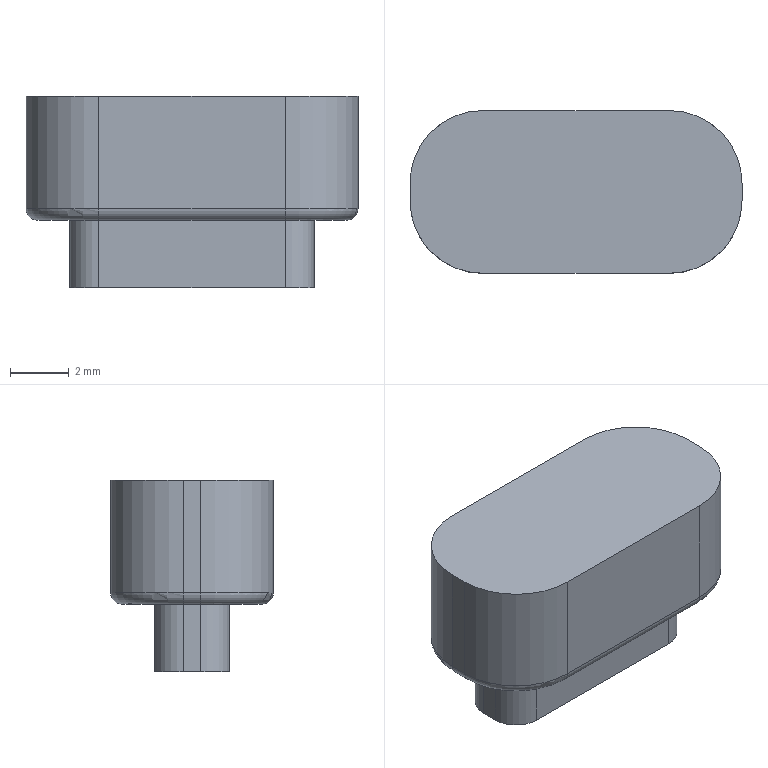Part | Creo | 1 solid | 27 faces | box 11.34 x 5.56 x 6.53 mm | volume 290.585 mm3 | cylinder 12 | plane 11 | torus 4 | commonest cylinder face diameters 0.8 x4 1.96 x4 4.96 x4
STEP:
#1=CARTESIAN_POINT('',(0.,0.,0.));
#2=DIRECTION('',(0.,0.,1.));
#3=DIRECTION('',(1.,0.,0.));
#4=AXIS2_PLACEMENT_3D('',#1,#2,#3);
#5=CARTESIAN_POINT('',(14.105,3.73,-58.15));
#6=VERTEX_POINT('',#5);
#7=CARTESIAN_POINT('',(7.725,3.73,-58.15));
#8=VERTEX_POINT('',#7);
#9=CARTESIAN_POINT('',(14.105,3.73,-58.15));
#10=DIRECTION('',(-1.,0.,0.));
#11=VECTOR('',#10,6.38);
#12=LINE('',#9,#11);
#13=EDGE_CURVE('',#6,#8,#12,.T.);
#14=ORIENTED_EDGE('',*,*,#13,.F.);
#15=CARTESIAN_POINT('',(14.105,3.73,-54.32));
#16=VERTEX_POINT('',#15);
#17=CARTESIAN_POINT('',(14.105,3.73,-54.32));
#18=DIRECTION('',(0.,0.,-1.));
#19=VECTOR('',#18,3.83);
#20=LINE('',#17,#19);
#21=EDGE_CURVE('',#16,#6,#20,.T.);
#22=ORIENTED_EDGE('',*,*,#21,.F.);
#23=CARTESIAN_POINT('',(7.725,3.73,-54.32));
#24=VERTEX_POINT('',#23);
#25=CARTESIAN_POINT('',(14.105,3.73,-54.32));
#26=DIRECTION('',(-1.,0.,0.));
#27=VECTOR('',#26,6.38);
#28=LINE('',#25,#27);
#29=EDGE_CURVE('',#16,#24,#28,.T.);
#30=ORIENTED_EDGE('',*,*,#29,.T.);
#31=CARTESIAN_POINT('',(7.725,3.73,-58.15));
#32=DIRECTION('',(0.,0.,1.));
#33=VECTOR('',#32,3.83);
#34=LINE('',#31,#33);
#35=EDGE_CURVE('',#8,#24,#34,.T.);
#36=ORIENTED_EDGE('',*,*,#35,.F.);
#37=EDGE_LOOP('',(#14,#22,#30,#36));
#38=FACE_OUTER_BOUND('',#37,.F.);
#39=CARTESIAN_POINT('',(14.105,3.73,-58.55));
#40=DIRECTION('',(0.,1.,0.));
#41=DIRECTION('',(-1.,0.,0.));
#42=AXIS2_PLACEMENT_3D('',#39,#40,#41);
#43=PLANE('',#42);
#44=ADVANCED_FACE('',(#38),#43,.T.);
#45=CARTESIAN_POINT('',(7.725,3.33,-58.55));
#46=VERTEX_POINT('',#45);
#47=CARTESIAN_POINT('',(14.105,3.33,-58.55));
#48=VERTEX_POINT('',#47);
#49=CARTESIAN_POINT('',(7.725,3.33,-58.55));
#50=DIRECTION('',(1.,0.,0.));
#51=VECTOR('',#50,6.38);
#52=LINE('',#49,#51);
#53=EDGE_CURVE('',#46,#48,#52,.T.);
#54=ORIENTED_EDGE('',*,*,#53,.T.);
#55=CARTESIAN_POINT('',(14.105,3.33,-58.15));
#56=DIRECTION('',(-1.,0.,0.));
#57=DIRECTION('',(0.,1.,0.));
#58=AXIS2_PLACEMENT_3D('',#55,#56,#57);
#59=CIRCLE('',#58,0.4);
#60=EDGE_CURVE('',#6,#48,#59,.T.);
#61=ORIENTED_EDGE('',*,*,#60,.F.);
#62=ORIENTED_EDGE('',*,*,#13,.T.);
#63=CARTESIAN_POINT('',(7.725,3.33,-58.15));
#64=DIRECTION('',(1.,0.,0.));
#65=DIRECTION('',(0.,0.,-1.));
#66=AXIS2_PLACEMENT_3D('',#63,#64,#65);
#67=CIRCLE('',#66,0.4);
#68=EDGE_CURVE('',#46,#8,#67,.T.);
#69=ORIENTED_EDGE('',*,*,#68,.F.);
#70=EDGE_LOOP('',(#54,#61,#62,#69));
#71=FACE_OUTER_BOUND('',#70,.F.);
#72=CARTESIAN_POINT('',(7.681,3.33,-58.15));
#73=DIRECTION('',(1.,0.,0.));
#74=DIRECTION('',(0.,0.,-1.));
#75=AXIS2_PLACEMENT_3D('',#72,#73,#74);
#76=CYLINDRICAL_SURFACE('',#75,0.4);
#77=ADVANCED_FACE('',(#71),#76,.T.);
#78=CARTESIAN_POINT('',(16.185,1.25,-58.55));
#79=VERTEX_POINT('',#78);
#80=CARTESIAN_POINT('',(14.105,1.25,-58.55));
#81=DIRECTION('',(0.,0.,1.));
#82=DIRECTION('',(1.,0.,0.));
#83=AXIS2_PLACEMENT_3D('',#80,#81,#82);
#84=CIRCLE('',#83,2.08);
#85=EDGE_CURVE('',#79,#48,#84,.T.);
#86=ORIENTED_EDGE('',*,*,#85,.T.);
#87=ORIENTED_EDGE('',*,*,#53,.F.);
#88=CARTESIAN_POINT('',(5.645,1.25,-58.55));
#89=VERTEX_POINT('',#88);
#90=CARTESIAN_POINT('',(7.725,1.25,-58.55));
#91=DIRECTION('',(0.,0.,1.));
#92=DIRECTION('',(0.,1.,0.));
#93=AXIS2_PLACEMENT_3D('',#90,#91,#92);
#94=CIRCLE('',#93,2.08);
#95=EDGE_CURVE('',#46,#89,#94,.T.);
#96=ORIENTED_EDGE('',*,*,#95,.T.);
#97=CARTESIAN_POINT('',(5.645,0.65,-58.55));
#98=VERTEX_POINT('',#97);
#99=CARTESIAN_POINT('',(5.645,0.65,-58.55));
#100=DIRECTION('',(0.,1.,0.));
#101=VECTOR('',#100,0.6);
#102=LINE('',#99,#101);
#103=EDGE_CURVE('',#98,#89,#102,.T.);
#104=ORIENTED_EDGE('',*,*,#103,.F.);
#105=CARTESIAN_POINT('',(7.725,-1.43,-58.55));
#106=VERTEX_POINT('',#105);
#107=CARTESIAN_POINT('',(7.725,0.65,-58.55));
#108=DIRECTION('',(0.,0.,1.));
#109=DIRECTION('',(-1.,0.,0.));
#110=AXIS2_PLACEMENT_3D('',#107,#108,#109);
#111=CIRCLE('',#110,2.08);
#112=EDGE_CURVE('',#98,#106,#111,.T.);
#113=ORIENTED_EDGE('',*,*,#112,.T.);
#114=CARTESIAN_POINT('',(14.105,-1.43,-58.55));
#115=VERTEX_POINT('',#114);
#116=CARTESIAN_POINT('',(14.105,-1.43,-58.55));
#117=DIRECTION('',(-1.,0.,0.));
#118=VECTOR('',#117,6.38);
#119=LINE('',#116,#118);
#120=EDGE_CURVE('',#115,#106,#119,.T.);
#121=ORIENTED_EDGE('',*,*,#120,.F.);
#122=CARTESIAN_POINT('',(16.185,0.65,-58.55));
#123=VERTEX_POINT('',#122);
#124=CARTESIAN_POINT('',(14.105,0.65,-58.55));
#125=DIRECTION('',(0.,0.,1.));
#126=DIRECTION('',(0.,-1.,0.));
#127=AXIS2_PLACEMENT_3D('',#124,#125,#126);
#128=CIRCLE('',#127,2.08);
#129=EDGE_CURVE('',#115,#123,#128,.T.);
#130=ORIENTED_EDGE('',*,*,#129,.T.);
#131=CARTESIAN_POINT('',(16.185,1.25,-58.55));
#132=DIRECTION('',(0.,-1.,0.));
#133=VECTOR('',#132,0.6);
#134=LINE('',#131,#133);
#135=EDGE_CURVE('',#79,#123,#134,.T.);
#136=ORIENTED_EDGE('',*,*,#135,.F.);
#137=EDGE_LOOP('',(#86,#87,#96,#104,#113,#121,#130,#136));
#138=FACE_OUTER_BOUND('',#137,.F.);
#139=CARTESIAN_POINT('',(15.085,0.65,-58.55));
#140=VERTEX_POINT('',#139);
#141=CARTESIAN_POINT('',(14.105,-0.33,-58.55));
#142=VERTEX_POINT('',#141);
#143=CARTESIAN_POINT('',(14.105,0.65,-58.55));
#144=DIRECTION('',(0.,0.,-1.));
#145=DIRECTION('',(1.,0.,0.));
#146=AXIS2_PLACEMENT_3D('',#143,#144,#145);
#147=CIRCLE('',#146,0.98);
#148=EDGE_CURVE('',#140,#142,#147,.T.);
#149=ORIENTED_EDGE('',*,*,#148,.T.);
#150=CARTESIAN_POINT('',(7.725,-0.33,-58.55));
#151=VERTEX_POINT('',#150);
#152=CARTESIAN_POINT('',(7.725,-0.33,-58.55));
#153=DIRECTION('',(1.,0.,0.));
#154=VECTOR('',#153,6.38);
#155=LINE('',#152,#154);
#156=EDGE_CURVE('',#151,#142,#155,.T.);
#157=ORIENTED_EDGE('',*,*,#156,.F.);
#158=CARTESIAN_POINT('',(6.745,0.65,-58.55));
#159=VERTEX_POINT('',#158);
#160=CARTESIAN_POINT('',(7.725,0.65,-58.55));
#161=DIRECTION('',(0.,0.,-1.));
#162=DIRECTION('',(0.,-1.,0.));
#163=AXIS2_PLACEMENT_3D('',#160,#161,#162);
#164=CIRCLE('',#163,0.98);
#165=EDGE_CURVE('',#151,#159,#164,.T.);
#166=ORIENTED_EDGE('',*,*,#165,.T.);
#167=CARTESIAN_POINT('',(6.745,1.25,-58.55));
#168=VERTEX_POINT('',#167);
#169=CARTESIAN_POINT('',(6.745,1.25,-58.55));
#170=DIRECTION('',(0.,-1.,0.));
#171=VECTOR('',#170,0.6);
#172=LINE('',#169,#171);
#173=EDGE_CURVE('',#168,#159,#172,.T.);
#174=ORIENTED_EDGE('',*,*,#173,.F.);
#175=CARTESIAN_POINT('',(7.725,2.23,-58.55));
#176=VERTEX_POINT('',#175);
#177=CARTESIAN_POINT('',(7.725,1.25,-58.55));
#178=DIRECTION('',(0.,0.,-1.));
#179=DIRECTION('',(-1.,0.,0.));
#180=AXIS2_PLACEMENT_3D('',#177,#178,#179);
#181=CIRCLE('',#180,0.98);
#182=EDGE_CURVE('',#168,#176,#181,.T.);
#183=ORIENTED_EDGE('',*,*,#182,.T.);
#184=CARTESIAN_POINT('',(14.105,2.23,-58.55));
#185=VERTEX_POINT('',#184);
#186=CARTESIAN_POINT('',(14.105,2.23,-58.55));
#187=DIRECTION('',(-1.,0.,0.));
#188=VECTOR('',#187,6.38);
#189=LINE('',#186,#188);
#190=EDGE_CURVE('',#185,#176,#189,.T.);
#191=ORIENTED_EDGE('',*,*,#190,.F.);
#192=CARTESIAN_POINT('',(15.085,1.25,-58.55));
#193=VERTEX_POINT('',#192);
#194=CARTESIAN_POINT('',(14.105,1.25,-58.55));
#195=DIRECTION('',(0.,0.,-1.));
#196=DIRECTION('',(0.,1.,0.));
#197=AXIS2_PLACEMENT_3D('',#194,#195,#196);
#198=CIRCLE('',#197,0.98);
#199=EDGE_CURVE('',#185,#193,#198,.T.);
#200=ORIENTED_EDGE('',*,*,#199,.T.);
#201=CARTESIAN_POINT('',(15.085,0.65,-58.55));
#202=DIRECTION('',(0.,1.,0.));
#203=VECTOR('',#202,0.6);
#204=LINE('',#201,#203);
#205=EDGE_CURVE('',#140,#193,#204,.T.);
#206=ORIENTED_EDGE('',*,*,#205,.F.);
#207=EDGE_LOOP('',(#149,#157,#166,#174,#183,#191,#200,#206));
#208=FACE_BOUND('',#207,.F.);
#209=CARTESIAN_POINT('',(0.,0.,-58.55));
#210=DIRECTION('',(0.,0.,1.));
#211=DIRECTION('',(1.,0.,0.));
#212=AXIS2_PLACEMENT_3D('',#209,#210,#211);
#213=PLANE('',#212);
#214=ADVANCED_FACE('',(#138,#208),#213,.F.);
#215=ORIENTED_EDGE('',*,*,#85,.F.);
#216=CARTESIAN_POINT('',(16.585,1.25,-58.15));
#217=VERTEX_POINT('',#216);
#218=CARTESIAN_POINT('',(16.185,1.25,-58.15));
#219=DIRECTION('',(0.,-1.,0.));
#220=DIRECTION('',(0.,0.,-1.));
#221=AXIS2_PLACEMENT_3D('',#218,#219,#220);
#222=CIRCLE('',#221,0.4);
#223=EDGE_CURVE('',#79,#217,#222,.T.);
#224=ORIENTED_EDGE('',*,*,#223,.T.);
#225=CARTESIAN_POINT('',(14.105,1.25,-58.15));
#226=DIRECTION('',(0.,0.,1.));
#227=DIRECTION('',(1.,0.,0.));
#228=AXIS2_PLACEMENT_3D('',#225,#226,#227);
#229=CIRCLE('',#228,2.48);
#230=EDGE_CURVE('',#217,#6,#229,.T.);
#231=ORIENTED_EDGE('',*,*,#230,.T.);
#232=ORIENTED_EDGE('',*,*,#60,.T.);
#233=EDGE_LOOP('',(#215,#224,#231,#232));
#234=FACE_OUTER_BOUND('',#233,.F.);
#235=CARTESIAN_POINT('',(14.105,1.25,-58.15));
#236=DIRECTION('',(0.,0.,1.));
#237=DIRECTION('',(-0.01768,0.9998,0.));
#238=AXIS2_PLACEMENT_3D('',#235,#236,#237);
#239=TOROIDAL_SURFACE('',#238,2.08,0.4);
#240=ADVANCED_FACE('',(#234),#239,.T.);
#241=ORIENTED_EDGE('',*,*,#135,.T.);
#242=CARTESIAN_POINT('',(16.585,0.65,-58.15));
#243=VERTEX_POINT('',#242);
#244=CARTESIAN_POINT('',(16.185,0.65,-58.15));
#245=DIRECTION('',(0.,1.,0.));
#246=DIRECTION('',(1.,0.,0.));
#247=AXIS2_PLACEMENT_3D('',#244,#245,#246);
#248=CIRCLE('',#247,0.4);
#249=EDGE_CURVE('',#243,#123,#248,.T.);
#250=ORIENTED_EDGE('',*,*,#249,.F.);
#251=CARTESIAN_POINT('',(16.585,0.65,-58.15));
#252=DIRECTION('',(0.,1.,0.));
#253=VECTOR('',#252,0.6);
#254=LINE('',#251,#253);
#255=EDGE_CURVE('',#243,#217,#254,.T.);
#256=ORIENTED_EDGE('',*,*,#255,.T.);
#257=ORIENTED_EDGE('',*,*,#223,.F.);
#258=EDGE_LOOP('',(#241,#250,#256,#257));
#259=FACE_OUTER_BOUND('',#258,.F.);
#260=CARTESIAN_POINT('',(16.185,1.294,-58.15));
#261=DIRECTION('',(0.,-1.,0.));
#262=DIRECTION('',(0.,0.,-1.));
#263=AXIS2_PLACEMENT_3D('',#260,#261,#262);
#264=CYLINDRICAL_SURFACE('',#263,0.4);
#265=ADVANCED_FACE('',(#259),#264,.T.);
#266=ORIENTED_EDGE('',*,*,#129,.F.);
#267=CARTESIAN_POINT('',(14.105,-1.83,-58.15));
#268=VERTEX_POINT('',#267);
#269=CARTESIAN_POINT('',(14.105,-1.43,-58.15));
#270=DIRECTION('',(-1.,0.,0.));
#271=DIRECTION('',(0.,0.,-1.));
#272=AXIS2_PLACEMENT_3D('',#269,#270,#271);
#273=CIRCLE('',#272,0.4);
#274=EDGE_CURVE('',#115,#268,#273,.T.);
#275=ORIENTED_EDGE('',*,*,#274,.T.);
#276=CARTESIAN_POINT('',(14.105,0.65,-58.15));
#277=DIRECTION('',(0.,0.,1.));
#278=DIRECTION('',(0.,-1.,0.));
#279=AXIS2_PLACEMENT_3D('',#276,#277,#278);
#280=CIRCLE('',#279,2.48);
#281=EDGE_CURVE('',#268,#243,#280,.T.);
#282=ORIENTED_EDGE('',*,*,#281,.T.);
#283=ORIENTED_EDGE('',*,*,#249,.T.);
#284=EDGE_LOOP('',(#266,#275,#282,#283));
#285=FACE_OUTER_BOUND('',#284,.F.);
#286=CARTESIAN_POINT('',(14.105,0.65,-58.15));
#287=DIRECTION('',(0.,0.,1.));
#288=DIRECTION('',(0.9998,0.01768,0.));
#289=AXIS2_PLACEMENT_3D('',#286,#287,#288);
#290=TOROIDAL_SURFACE('',#289,2.08,0.4);
#291=ADVANCED_FACE('',(#285),#290,.T.);
#292=ORIENTED_EDGE('',*,*,#120,.T.);
#293=CARTESIAN_POINT('',(7.725,-1.83,-58.15));
#294=VERTEX_POINT('',#293);
#295=CARTESIAN_POINT('',(7.725,-1.43,-58.15));
#296=DIRECTION('',(1.,0.,0.));
#297=DIRECTION('',(0.,-1.,0.));
#298=AXIS2_PLACEMENT_3D('',#295,#296,#297);
#299=CIRCLE('',#298,0.4);
#300=EDGE_CURVE('',#294,#106,#299,.T.);
#301=ORIENTED_EDGE('',*,*,#300,.F.);
#302=CARTESIAN_POINT('',(7.725,-1.83,-58.15));
#303=DIRECTION('',(1.,0.,0.));
#304=VECTOR('',#303,6.38);
#305=LINE('',#302,#304);
#306=EDGE_CURVE('',#294,#268,#305,.T.);
#307=ORIENTED_EDGE('',*,*,#306,.T.);
#308=ORIENTED_EDGE('',*,*,#274,.F.);
#309=EDGE_LOOP('',(#292,#301,#307,#308));
#310=FACE_OUTER_BOUND('',#309,.F.);
#311=CARTESIAN_POINT('',(14.149,-1.43,-58.15));
#312=DIRECTION('',(-1.,0.,0.));
#313=DIRECTION('',(0.,0.,-1.));
#314=AXIS2_PLACEMENT_3D('',#311,#312,#313);
#315=CYLINDRICAL_SURFACE('',#314,0.4);
#316=ADVANCED_FACE('',(#310),#315,.T.);
#317=ORIENTED_EDGE('',*,*,#112,.F.);
#318=CARTESIAN_POINT('',(5.245,0.65,-58.15));
#319=VERTEX_POINT('',#318);
#320=CARTESIAN_POINT('',(5.645,0.65,-58.15));
#321=DIRECTION('',(0.,1.,0.));
#322=DIRECTION('',(0.,0.,-1.));
#323=AXIS2_PLACEMENT_3D('',#320,#321,#322);
#324=CIRCLE('',#323,0.4);
#325=EDGE_CURVE('',#98,#319,#324,.T.);
#326=ORIENTED_EDGE('',*,*,#325,.T.);
#327=CARTESIAN_POINT('',(7.725,0.65,-58.15));
#328=DIRECTION('',(0.,0.,1.));
#329=DIRECTION('',(-1.,0.,0.));
#330=AXIS2_PLACEMENT_3D('',#327,#328,#329);
#331=CIRCLE('',#330,2.48);
#332=EDGE_CURVE('',#319,#294,#331,.T.);
#333=ORIENTED_EDGE('',*,*,#332,.T.);
#334=ORIENTED_EDGE('',*,*,#300,.T.);
#335=EDGE_LOOP('',(#317,#326,#333,#334));
#336=FACE_OUTER_BOUND('',#335,.F.);
#337=CARTESIAN_POINT('',(7.725,0.65,-58.15));
#338=DIRECTION('',(0.,0.,1.));
#339=DIRECTION('',(0.01768,-0.9998,0.));
#340=AXIS2_PLACEMENT_3D('',#337,#338,#339);
#341=TOROIDAL_SURFACE('',#340,2.08,0.4);
#342=ADVANCED_FACE('',(#336),#341,.T.);
#343=ORIENTED_EDGE('',*,*,#103,.T.);
#344=CARTESIAN_POINT('',(5.245,1.25,-58.15));
#345=VERTEX_POINT('',#344);
#346=CARTESIAN_POINT('',(5.645,1.25,-58.15));
#347=DIRECTION('',(0.,-1.,0.));
#348=DIRECTION('',(-1.,0.,0.));
#349=AXIS2_PLACEMENT_3D('',#346,#347,#348);
#350=CIRCLE('',#349,0.4);
#351=EDGE_CURVE('',#345,#89,#350,.T.);
#352=ORIENTED_EDGE('',*,*,#351,.F.);
#353=CARTESIAN_POINT('',(5.245,1.25,-58.15));
#354=DIRECTION('',(0.,-1.,0.));
#355=VECTOR('',#354,0.6);
#356=LINE('',#353,#355);
#357=EDGE_CURVE('',#345,#319,#356,.T.);
#358=ORIENTED_EDGE('',*,*,#357,.T.);
#359=ORIENTED_EDGE('',*,*,#325,.F.);
#360=EDGE_LOOP('',(#343,#352,#358,#359));
#361=FACE_OUTER_BOUND('',#360,.F.);
#362=CARTESIAN_POINT('',(5.645,0.6062,-58.15));
#363=DIRECTION('',(0.,1.,0.));
#364=DIRECTION('',(0.,0.,-1.));
#365=AXIS2_PLACEMENT_3D('',#362,#363,#364);
#366=CYLINDRICAL_SURFACE('',#365,0.4);
#367=ADVANCED_FACE('',(#361),#366,.T.);
#368=ORIENTED_EDGE('',*,*,#95,.F.);
#369=ORIENTED_EDGE('',*,*,#68,.T.);
#370=CARTESIAN_POINT('',(7.725,1.25,-58.15));
#371=DIRECTION('',(0.,0.,1.));
#372=DIRECTION('',(0.,1.,0.));
#373=AXIS2_PLACEMENT_3D('',#370,#371,#372);
#374=CIRCLE('',#373,2.48);
#375=EDGE_CURVE('',#8,#345,#374,.T.);
#376=ORIENTED_EDGE('',*,*,#375,.T.);
#377=ORIENTED_EDGE('',*,*,#351,.T.);
#378=EDGE_LOOP('',(#368,#369,#376,#377));
#379=FACE_OUTER_BOUND('',#378,.F.);
#380=CARTESIAN_POINT('',(7.725,1.25,-58.15));
#381=DIRECTION('',(0.,0.,1.));
#382=DIRECTION('',(-0.9998,-0.01768,0.));
#383=AXIS2_PLACEMENT_3D('',#380,#381,#382);
#384=TOROIDAL_SURFACE('',#383,2.08,0.4);
#385=ADVANCED_FACE('',(#379),#384,.T.);
#386=ORIENTED_EDGE('',*,*,#375,.F.);
#387=ORIENTED_EDGE('',*,*,#35,.T.);
#388=CARTESIAN_POINT('',(5.245,1.25,-54.32));
#389=VERTEX_POINT('',#388);
#390=CARTESIAN_POINT('',(7.725,1.25,-54.32));
#391=DIRECTION('',(0.,0.,-1.));
#392=DIRECTION('',(-1.,0.,0.));
#393=AXIS2_PLACEMENT_3D('',#390,#391,#392);
#394=CIRCLE('',#393,2.48);
#395=EDGE_CURVE('',#389,#24,#394,.T.);
#396=ORIENTED_EDGE('',*,*,#395,.F.);
#397=CARTESIAN_POINT('',(5.245,1.25,-54.32));
#398=DIRECTION('',(0.,0.,-1.));
#399=VECTOR('',#398,3.83);
#400=LINE('',#397,#399);
#401=EDGE_CURVE('',#389,#345,#400,.T.);
#402=ORIENTED_EDGE('',*,*,#401,.T.);
#403=EDGE_LOOP('',(#386,#387,#396,#402));
#404=FACE_OUTER_BOUND('',#403,.F.);
#405=CARTESIAN_POINT('',(7.725,1.25,-58.55));
#406=DIRECTION('',(0.,0.,1.));
#407=DIRECTION('',(1.,0.,0.));
#408=AXIS2_PLACEMENT_3D('',#405,#406,#407);
#409=CYLINDRICAL_SURFACE('',#408,2.48);
#410=ADVANCED_FACE('',(#404),#409,.T.);
#411=CARTESIAN_POINT('',(16.585,0.65,-54.32));
#412=VERTEX_POINT('',#411);
#413=CARTESIAN_POINT('',(14.105,-1.83,-54.32));
#414=VERTEX_POINT('',#413);
#415=CARTESIAN_POINT('',(14.105,0.65,-54.32));
#416=DIRECTION('',(0.,0.,-1.));
#417=DIRECTION('',(1.,0.,0.));
#418=AXIS2_PLACEMENT_3D('',#415,#416,#417);
#419=CIRCLE('',#418,2.48);
#420=EDGE_CURVE('',#412,#414,#419,.T.);
#421=ORIENTED_EDGE('',*,*,#420,.T.);
#422=CARTESIAN_POINT('',(7.725,-1.83,-54.32));
#423=VERTEX_POINT('',#422);
#424=CARTESIAN_POINT('',(7.725,-1.83,-54.32));
#425=DIRECTION('',(1.,0.,0.));
#426=VECTOR('',#425,6.38);
#427=LINE('',#424,#426);
#428=EDGE_CURVE('',#423,#414,#427,.T.);
#429=ORIENTED_EDGE('',*,*,#428,.F.);
#430=CARTESIAN_POINT('',(5.245,0.65,-54.32));
#431=VERTEX_POINT('',#430);
#432=CARTESIAN_POINT('',(7.725,0.65,-54.32));
#433=DIRECTION('',(0.,0.,-1.));
#434=DIRECTION('',(0.,-1.,0.));
#435=AXIS2_PLACEMENT_3D('',#432,#433,#434);
#436=CIRCLE('',#435,2.48);
#437=EDGE_CURVE('',#423,#431,#436,.T.);
#438=ORIENTED_EDGE('',*,*,#437,.T.);
#439=CARTESIAN_POINT('',(5.245,1.25,-54.32));
#440=DIRECTION('',(0.,-1.,0.));
#441=VECTOR('',#440,0.6);
#442=LINE('',#439,#441);
#443=EDGE_CURVE('',#389,#431,#442,.T.);
#444=ORIENTED_EDGE('',*,*,#443,.F.);
#445=ORIENTED_EDGE('',*,*,#395,.T.);
#446=ORIENTED_EDGE('',*,*,#29,.F.);
#447=CARTESIAN_POINT('',(16.585,1.25,-54.32));
#448=VERTEX_POINT('',#447);
#449=CARTESIAN_POINT('',(14.105,1.25,-54.32));
#450=DIRECTION('',(0.,0.,-1.));
#451=DIRECTION('',(0.,1.,0.));
#452=AXIS2_PLACEMENT_3D('',#449,#450,#451);
#453=CIRCLE('',#452,2.48);
#454=EDGE_CURVE('',#16,#448,#453,.T.);
#455=ORIENTED_EDGE('',*,*,#454,.T.);
#456=CARTESIAN_POINT('',(16.585,0.65,-54.32));
#457=DIRECTION('',(0.,1.,0.));
#458=VECTOR('',#457,0.6);
#459=LINE('',#456,#458);
#460=EDGE_CURVE('',#412,#448,#459,.T.);
#461=ORIENTED_EDGE('',*,*,#460,.F.);
#462=EDGE_LOOP('',(#421,#429,#438,#444,#445,#446,#455,#461));
#463=FACE_OUTER_BOUND('',#462,.F.);
#464=CARTESIAN_POINT('',(0.,0.,-54.32));
#465=DIRECTION('',(0.,0.,1.));
#466=DIRECTION('',(1.,0.,0.));
#467=AXIS2_PLACEMENT_3D('',#464,#465,#466);
#468=PLANE('',#467);
#469=ADVANCED_FACE('',(#463),#468,.T.);
#470=ORIENTED_EDGE('',*,*,#281,.F.);
#471=CARTESIAN_POINT('',(14.105,-1.83,-58.15));
#472=DIRECTION('',(0.,0.,1.));
#473=VECTOR('',#472,3.83);
#474=LINE('',#471,#473);
#475=EDGE_CURVE('',#268,#414,#474,.T.);
#476=ORIENTED_EDGE('',*,*,#475,.T.);
#477=ORIENTED_EDGE('',*,*,#420,.F.);
#478=CARTESIAN_POINT('',(16.585,0.65,-54.32));
#479=DIRECTION('',(0.,0.,-1.));
#480=VECTOR('',#479,3.83);
#481=LINE('',#478,#480);
#482=EDGE_CURVE('',#412,#243,#481,.T.);
#483=ORIENTED_EDGE('',*,*,#482,.T.);
#484=EDGE_LOOP('',(#470,#476,#477,#483));
#485=FACE_OUTER_BOUND('',#484,.F.);
#486=CARTESIAN_POINT('',(14.105,0.65,-58.55));
#487=DIRECTION('',(0.,0.,1.));
#488=DIRECTION('',(1.,0.,0.));
#489=AXIS2_PLACEMENT_3D('',#486,#487,#488);
#490=CYLINDRICAL_SURFACE('',#489,2.48);
#491=ADVANCED_FACE('',(#485),#490,.T.);
#492=ORIENTED_EDGE('',*,*,#306,.F.);
#493=CARTESIAN_POINT('',(7.725,-1.83,-54.32));
#494=DIRECTION('',(0.,0.,-1.));
#495=VECTOR('',#494,3.83);
#496=LINE('',#493,#495);
#497=EDGE_CURVE('',#423,#294,#496,.T.);
#498=ORIENTED_EDGE('',*,*,#497,.F.);
#499=ORIENTED_EDGE('',*,*,#428,.T.);
#500=ORIENTED_EDGE('',*,*,#475,.F.);
#501=EDGE_LOOP('',(#492,#498,#499,#500));
#502=FACE_OUTER_BOUND('',#501,.F.);
#503=CARTESIAN_POINT('',(7.725,-1.83,-58.55));
#504=DIRECTION('',(0.,-1.,0.));
#505=DIRECTION('',(1.,0.,0.));
#506=AXIS2_PLACEMENT_3D('',#503,#504,#505);
#507=PLANE('',#506);
#508=ADVANCED_FACE('',(#502),#507,.T.);
#509=ORIENTED_EDGE('',*,*,#332,.F.);
#510=CARTESIAN_POINT('',(5.245,0.65,-58.15));
#511=DIRECTION('',(0.,0.,1.));
#512=VECTOR('',#511,3.83);
#513=LINE('',#510,#512);
#514=EDGE_CURVE('',#319,#431,#513,.T.);
#515=ORIENTED_EDGE('',*,*,#514,.T.);
#516=ORIENTED_EDGE('',*,*,#437,.F.);
#517=ORIENTED_EDGE('',*,*,#497,.T.);
#518=EDGE_LOOP('',(#509,#515,#516,#517));
#519=FACE_OUTER_BOUND('',#518,.F.);
#520=CARTESIAN_POINT('',(7.725,0.65,-58.55));
#521=DIRECTION('',(0.,0.,1.));
#522=DIRECTION('',(1.,0.,0.));
#523=AXIS2_PLACEMENT_3D('',#520,#521,#522);
#524=CYLINDRICAL_SURFACE('',#523,2.48);
#525=ADVANCED_FACE('',(#519),#524,.T.);
#526=ORIENTED_EDGE('',*,*,#357,.F.);
#527=ORIENTED_EDGE('',*,*,#401,.F.);
#528=ORIENTED_EDGE('',*,*,#443,.T.);
#529=ORIENTED_EDGE('',*,*,#514,.F.);
#530=EDGE_LOOP('',(#526,#527,#528,#529));
#531=FACE_OUTER_BOUND('',#530,.F.);
#532=CARTESIAN_POINT('',(5.245,1.25,-58.55));
#533=DIRECTION('',(-1.,0.,0.));
#534=DIRECTION('',(0.,-1.,0.));
#535=AXIS2_PLACEMENT_3D('',#532,#533,#534);
#536=PLANE('',#535);
#537=ADVANCED_FACE('',(#531),#536,.T.);
#538=ORIENTED_EDGE('',*,*,#255,.F.);
#539=ORIENTED_EDGE('',*,*,#482,.F.);
#540=ORIENTED_EDGE('',*,*,#460,.T.);
#541=CARTESIAN_POINT('',(16.585,1.25,-58.15));
#542=DIRECTION('',(0.,0.,1.));
#543=VECTOR('',#542,3.83);
#544=LINE('',#541,#543);
#545=EDGE_CURVE('',#217,#448,#544,.T.);
#546=ORIENTED_EDGE('',*,*,#545,.F.);
#547=EDGE_LOOP('',(#538,#539,#540,#546));
#548=FACE_OUTER_BOUND('',#547,.F.);
#549=CARTESIAN_POINT('',(16.585,0.65,-58.55));
#550=DIRECTION('',(1.,0.,0.));
#551=DIRECTION('',(0.,1.,0.));
#552=AXIS2_PLACEMENT_3D('',#549,#550,#551);
#553=PLANE('',#552);
#554=ADVANCED_FACE('',(#548),#553,.T.);
#555=ORIENTED_EDGE('',*,*,#230,.F.);
#556=ORIENTED_EDGE('',*,*,#545,.T.);
#557=ORIENTED_EDGE('',*,*,#454,.F.);
#558=ORIENTED_EDGE('',*,*,#21,.T.);
#559=EDGE_LOOP('',(#555,#556,#557,#558));
#560=FACE_OUTER_BOUND('',#559,.F.);
#561=CARTESIAN_POINT('',(14.105,1.25,-58.55));
#562=DIRECTION('',(0.,0.,1.));
#563=DIRECTION('',(1.,0.,0.));
#564=AXIS2_PLACEMENT_3D('',#561,#562,#563);
#565=CYLINDRICAL_SURFACE('',#564,2.48);
#566=ADVANCED_FACE('',(#560),#565,.T.);
#567=ORIENTED_EDGE('',*,*,#148,.F.);
#568=CARTESIAN_POINT('',(15.085,0.65,-60.85));
#569=VERTEX_POINT('',#568);
#570=CARTESIAN_POINT('',(15.085,0.65,-58.55));
#571=DIRECTION('',(0.,0.,-1.));
#572=VECTOR('',#571,2.3);
#573=LINE('',#570,#572);
#574=EDGE_CURVE('',#140,#569,#573,.T.);
#575=ORIENTED_EDGE('',*,*,#574,.T.);
#576=CARTESIAN_POINT('',(14.105,-0.33,-60.85));
#577=VERTEX_POINT('',#576);
#578=CARTESIAN_POINT('',(14.105,0.65,-60.85));
#579=DIRECTION('',(0.,0.,1.));
#580=DIRECTION('',(0.,-1.,0.));
#581=AXIS2_PLACEMENT_3D('',#578,#579,#580);
#582=CIRCLE('',#581,0.98);
#583=EDGE_CURVE('',#577,#569,#582,.T.);
#584=ORIENTED_EDGE('',*,*,#583,.F.);
#585=CARTESIAN_POINT('',(14.105,-0.33,-60.85));
#586=DIRECTION('',(0.,0.,1.));
#587=VECTOR('',#586,2.3);
#588=LINE('',#585,#587);
#589=EDGE_CURVE('',#577,#142,#588,.T.);
#590=ORIENTED_EDGE('',*,*,#589,.T.);
#591=EDGE_LOOP('',(#567,#575,#584,#590));
#592=FACE_OUTER_BOUND('',#591,.F.);
#593=CARTESIAN_POINT('',(14.105,0.65,-60.85));
#594=DIRECTION('',(0.,0.,1.));
#595=DIRECTION('',(1.,0.,0.));
#596=AXIS2_PLACEMENT_3D('',#593,#594,#595);
#597=CYLINDRICAL_SURFACE('',#596,0.98);
#598=ADVANCED_FACE('',(#592),#597,.T.);
#599=ORIENTED_EDGE('',*,*,#205,.T.);
#600=CARTESIAN_POINT('',(15.085,1.25,-60.85));
#601=VERTEX_POINT('',#600);
#602=CARTESIAN_POINT('',(15.085,1.25,-60.85));
#603=DIRECTION('',(0.,0.,1.));
#604=VECTOR('',#603,2.3);
#605=LINE('',#602,#604);
#606=EDGE_CURVE('',#601,#193,#605,.T.);
#607=ORIENTED_EDGE('',*,*,#606,.F.);
#608=CARTESIAN_POINT('',(15.085,0.65,-60.85));
#609=DIRECTION('',(0.,1.,0.));
#610=VECTOR('',#609,0.6);
#611=LINE('',#608,#610);
#612=EDGE_CURVE('',#569,#601,#611,.T.);
#613=ORIENTED_EDGE('',*,*,#612,.F.);
#614=ORIENTED_EDGE('',*,*,#574,.F.);
#615=EDGE_LOOP('',(#599,#607,#613,#614));
#616=FACE_OUTER_BOUND('',#615,.F.);
#617=CARTESIAN_POINT('',(15.085,0.65,-60.85));
#618=DIRECTION('',(1.,0.,0.));
#619=DIRECTION('',(0.,1.,0.));
#620=AXIS2_PLACEMENT_3D('',#617,#618,#619);
#621=PLANE('',#620);
#622=ADVANCED_FACE('',(#616),#621,.T.);
#623=ORIENTED_EDGE('',*,*,#199,.F.);
#624=CARTESIAN_POINT('',(14.105,2.23,-60.85));
#625=VERTEX_POINT('',#624);
#626=CARTESIAN_POINT('',(14.105,2.23,-58.55));
#627=DIRECTION('',(0.,0.,-1.));
#628=VECTOR('',#627,2.3);
#629=LINE('',#626,#628);
#630=EDGE_CURVE('',#185,#625,#629,.T.);
#631=ORIENTED_EDGE('',*,*,#630,.T.);
#632=CARTESIAN_POINT('',(14.105,1.25,-60.85));
#633=DIRECTION('',(0.,0.,1.));
#634=DIRECTION('',(1.,0.,0.));
#635=AXIS2_PLACEMENT_3D('',#632,#633,#634);
#636=CIRCLE('',#635,0.98);
#637=EDGE_CURVE('',#601,#625,#636,.T.);
#638=ORIENTED_EDGE('',*,*,#637,.F.);
#639=ORIENTED_EDGE('',*,*,#606,.T.);
#640=EDGE_LOOP('',(#623,#631,#638,#639));
#641=FACE_OUTER_BOUND('',#640,.F.);
#642=CARTESIAN_POINT('',(14.105,1.25,-60.85));
#643=DIRECTION('',(0.,0.,1.));
#644=DIRECTION('',(1.,0.,0.));
#645=AXIS2_PLACEMENT_3D('',#642,#643,#644);
#646=CYLINDRICAL_SURFACE('',#645,0.98);
#647=ADVANCED_FACE('',(#641),#646,.T.);
#648=ORIENTED_EDGE('',*,*,#190,.T.);
#649=CARTESIAN_POINT('',(7.725,2.23,-60.85));
#650=VERTEX_POINT('',#649);
#651=CARTESIAN_POINT('',(7.725,2.23,-60.85));
#652=DIRECTION('',(0.,0.,1.));
#653=VECTOR('',#652,2.3);
#654=LINE('',#651,#653);
#655=EDGE_CURVE('',#650,#176,#654,.T.);
#656=ORIENTED_EDGE('',*,*,#655,.F.);
#657=CARTESIAN_POINT('',(14.105,2.23,-60.85));
#658=DIRECTION('',(-1.,0.,0.));
#659=VECTOR('',#658,6.38);
#660=LINE('',#657,#659);
#661=EDGE_CURVE('',#625,#650,#660,.T.);
#662=ORIENTED_EDGE('',*,*,#661,.F.);
#663=ORIENTED_EDGE('',*,*,#630,.F.);
#664=EDGE_LOOP('',(#648,#656,#662,#663));
#665=FACE_OUTER_BOUND('',#664,.F.);
#666=CARTESIAN_POINT('',(14.105,2.23,-60.85));
#667=DIRECTION('',(0.,1.,0.));
#668=DIRECTION('',(-1.,0.,0.));
#669=AXIS2_PLACEMENT_3D('',#666,#667,#668);
#670=PLANE('',#669);
#671=ADVANCED_FACE('',(#665),#670,.T.);
#672=ORIENTED_EDGE('',*,*,#182,.F.);
#673=CARTESIAN_POINT('',(6.745,1.25,-60.85));
#674=VERTEX_POINT('',#673);
#675=CARTESIAN_POINT('',(6.745,1.25,-58.55));
#676=DIRECTION('',(0.,0.,-1.));
#677=VECTOR('',#676,2.3);
#678=LINE('',#675,#677);
#679=EDGE_CURVE('',#168,#674,#678,.T.);
#680=ORIENTED_EDGE('',*,*,#679,.T.);
#681=CARTESIAN_POINT('',(7.725,1.25,-60.85));
#682=DIRECTION('',(0.,0.,1.));
#683=DIRECTION('',(0.,1.,0.));
#684=AXIS2_PLACEMENT_3D('',#681,#682,#683);
#685=CIRCLE('',#684,0.98);
#686=EDGE_CURVE('',#650,#674,#685,.T.);
#687=ORIENTED_EDGE('',*,*,#686,.F.);
#688=ORIENTED_EDGE('',*,*,#655,.T.);
#689=EDGE_LOOP('',(#672,#680,#687,#688));
#690=FACE_OUTER_BOUND('',#689,.F.);
#691=CARTESIAN_POINT('',(7.725,1.25,-60.85));
#692=DIRECTION('',(0.,0.,1.));
#693=DIRECTION('',(1.,0.,0.));
#694=AXIS2_PLACEMENT_3D('',#691,#692,#693);
#695=CYLINDRICAL_SURFACE('',#694,0.98);
#696=ADVANCED_FACE('',(#690),#695,.T.);
#697=ORIENTED_EDGE('',*,*,#173,.T.);
#698=CARTESIAN_POINT('',(6.745,0.65,-60.85));
#699=VERTEX_POINT('',#698);
#700=CARTESIAN_POINT('',(6.745,0.65,-60.85));
#701=DIRECTION('',(0.,0.,1.));
#702=VECTOR('',#701,2.3);
#703=LINE('',#700,#702);
#704=EDGE_CURVE('',#699,#159,#703,.T.);
#705=ORIENTED_EDGE('',*,*,#704,.F.);
#706=CARTESIAN_POINT('',(6.745,1.25,-60.85));
#707=DIRECTION('',(0.,-1.,0.));
#708=VECTOR('',#707,0.6);
#709=LINE('',#706,#708);
#710=EDGE_CURVE('',#674,#699,#709,.T.);
#711=ORIENTED_EDGE('',*,*,#710,.F.);
#712=ORIENTED_EDGE('',*,*,#679,.F.);
#713=EDGE_LOOP('',(#697,#705,#711,#712));
#714=FACE_OUTER_BOUND('',#713,.F.);
#715=CARTESIAN_POINT('',(6.745,1.25,-60.85));
#716=DIRECTION('',(-1.,0.,0.));
#717=DIRECTION('',(0.,-1.,0.));
#718=AXIS2_PLACEMENT_3D('',#715,#716,#717);
#719=PLANE('',#718);
#720=ADVANCED_FACE('',(#714),#719,.T.);
#721=ORIENTED_EDGE('',*,*,#165,.F.);
#722=CARTESIAN_POINT('',(7.725,-0.33,-60.85));
#723=VERTEX_POINT('',#722);
#724=CARTESIAN_POINT('',(7.725,-0.33,-58.55));
#725=DIRECTION('',(0.,0.,-1.));
#726=VECTOR('',#725,2.3);
#727=LINE('',#724,#726);
#728=EDGE_CURVE('',#151,#723,#727,.T.);
#729=ORIENTED_EDGE('',*,*,#728,.T.);
#730=CARTESIAN_POINT('',(7.725,0.65,-60.85));
#731=DIRECTION('',(0.,0.,1.));
#732=DIRECTION('',(-1.,0.,0.));
#733=AXIS2_PLACEMENT_3D('',#730,#731,#732);
#734=CIRCLE('',#733,0.98);
#735=EDGE_CURVE('',#699,#723,#734,.T.);
#736=ORIENTED_EDGE('',*,*,#735,.F.);
#737=ORIENTED_EDGE('',*,*,#704,.T.);
#738=EDGE_LOOP('',(#721,#729,#736,#737));
#739=FACE_OUTER_BOUND('',#738,.F.);
#740=CARTESIAN_POINT('',(7.725,0.65,-60.85));
#741=DIRECTION('',(0.,0.,1.));
#742=DIRECTION('',(1.,0.,0.));
#743=AXIS2_PLACEMENT_3D('',#740,#741,#742);
#744=CYLINDRICAL_SURFACE('',#743,0.98);
#745=ADVANCED_FACE('',(#739),#744,.T.);
#746=ORIENTED_EDGE('',*,*,#156,.T.);
#747=ORIENTED_EDGE('',*,*,#589,.F.);
#748=CARTESIAN_POINT('',(7.725,-0.33,-60.85));
#749=DIRECTION('',(1.,0.,0.));
#750=VECTOR('',#749,6.38);
#751=LINE('',#748,#750);
#752=EDGE_CURVE('',#723,#577,#751,.T.);
#753=ORIENTED_EDGE('',*,*,#752,.F.);
#754=ORIENTED_EDGE('',*,*,#728,.F.);
#755=EDGE_LOOP('',(#746,#747,#753,#754));
#756=FACE_OUTER_BOUND('',#755,.F.);
#757=CARTESIAN_POINT('',(7.725,-0.33,-60.85));
#758=DIRECTION('',(0.,-1.,0.));
#759=DIRECTION('',(1.,0.,0.));
#760=AXIS2_PLACEMENT_3D('',#757,#758,#759);
#761=PLANE('',#760);
#762=ADVANCED_FACE('',(#756),#761,.T.);
#763=ORIENTED_EDGE('',*,*,#583,.T.);
#764=ORIENTED_EDGE('',*,*,#612,.T.);
#765=ORIENTED_EDGE('',*,*,#637,.T.);
#766=ORIENTED_EDGE('',*,*,#661,.T.);
#767=ORIENTED_EDGE('',*,*,#686,.T.);
#768=ORIENTED_EDGE('',*,*,#710,.T.);
#769=ORIENTED_EDGE('',*,*,#735,.T.);
#770=ORIENTED_EDGE('',*,*,#752,.T.);
#771=EDGE_LOOP('',(#763,#764,#765,#766,#767,#768,#769,#770));
#772=FACE_OUTER_BOUND('',#771,.F.);
#773=CARTESIAN_POINT('',(0.,0.,-60.85));
#774=DIRECTION('',(0.,0.,1.));
#775=DIRECTION('',(1.,0.,0.));
#776=AXIS2_PLACEMENT_3D('',#773,#774,#775);
#777=PLANE('',#776);
#778=ADVANCED_FACE('',(#772),#777,.F.);
#779=CLOSED_SHELL('',(#44,#77,#214,#240,#265,#291,#316,#342,#367,#385,#410,#469,#491,#508,#525,#537,#554,#566,#598,#622,#647,#671,#696,#720,#745,#762,#778));
#780=MANIFOLD_SOLID_BREP('',#779);
#781=(LENGTH_UNIT()NAMED_UNIT(*)SI_UNIT(.MILLI.,.METRE.));
#782=UNCERTAINTY_MEASURE_WITH_UNIT(LENGTH_MEASURE(0.001422),#781,'','');
#783=(NAMED_UNIT(*)PLANE_ANGLE_UNIT()SI_UNIT($,.RADIAN.));
#784=PLANE_ANGLE_MEASURE_WITH_UNIT(PLANE_ANGLE_MEASURE(0.01745),#783);
#785=(CONVERSION_BASED_UNIT('DEGREE',#784)NAMED_UNIT(*)PLANE_ANGLE_UNIT());
#786=(NAMED_UNIT(*)SI_UNIT($,.STERADIAN.)SOLID_ANGLE_UNIT());
#787=(GEOMETRIC_REPRESENTATION_CONTEXT(3)GLOBAL_UNCERTAINTY_ASSIGNED_CONTEXT((#782))GLOBAL_UNIT_ASSIGNED_CONTEXT((#781,#785,#786))REPRESENTATION_CONTEXT('',''));
#788=ADVANCED_BREP_SHAPE_REPRESENTATION('',(#4,#780),#787);